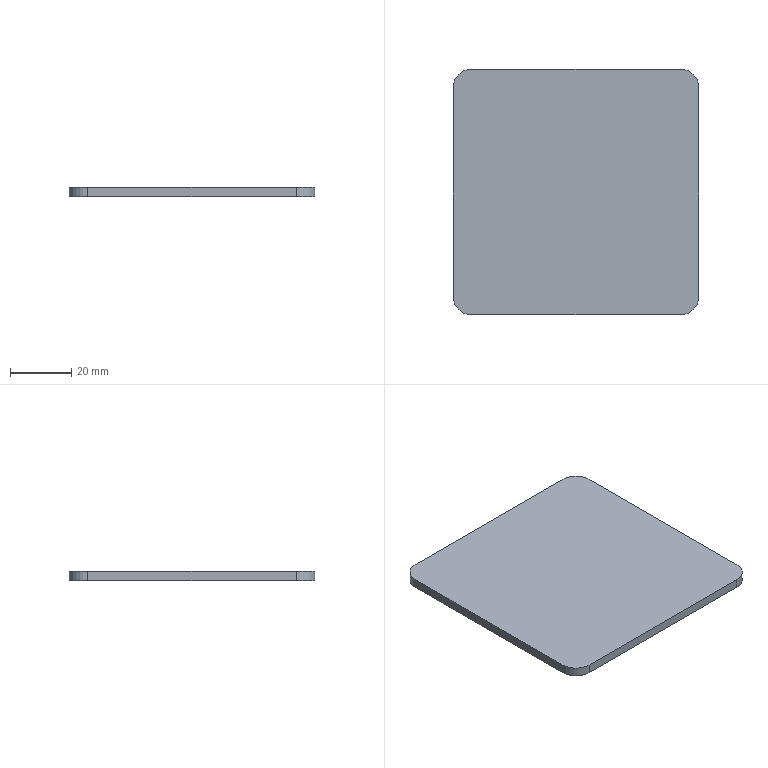Part | STEP file | SN10_008_006-04_TAMPA | 1 solid | 10 faces | box 80 x 80 x 3 mm | volume 19107 mm3 | plane 6 | cylinder 4 | commonest cylinder face diameters 12 x4
STEP:
#1=CARTESIAN_POINT('',(0.,0.,0.));
#2=DIRECTION('',(0.,0.,1.));
#3=DIRECTION('',(1.,0.,0.));
#4=AXIS2_PLACEMENT_3D('',#1,#2,#3);
#5=CARTESIAN_POINT('',(249.629,350.,449.));
#6=VERTEX_POINT('',#5);
#7=CARTESIAN_POINT('',(317.629,350.,449.));
#8=VERTEX_POINT('',#7);
#9=CARTESIAN_POINT('',(249.629,350.,449.));
#10=DIRECTION('',(1.,0.,0.));
#11=VECTOR('',#10,1.);
#12=LINE('',#9,#11);
#13=CARTESIAN_POINT('',(249.629,350.,446.));
#14=DIRECTION('',(0.,-1.,0.));
#15=DIRECTION('',(0.,0.,-1.));
#16=AXIS2_PLACEMENT_3D('',#13,#14,#15);
#17=PLANE('',#16);
#18=CARTESIAN_POINT('',(-3.,0.));
#19=DIRECTION('',(0.,1.));
#20=VECTOR('',#19,1.);
#21=LINE('',#18,#20);
#22=(GEOMETRIC_REPRESENTATION_CONTEXT(2)PARAMETRIC_REPRESENTATION_CONTEXT()REPRESENTATION_CONTEXT('',''));
#23=DEFINITIONAL_REPRESENTATION('',(#21),#22);
#24=PCURVE('',#17,#23);
#25=CARTESIAN_POINT('',(0.,0.,449.));
#26=DIRECTION('',(0.,0.,-1.));
#27=DIRECTION('',(-1.,0.,0.));
#28=AXIS2_PLACEMENT_3D('',#25,#26,#27);
#29=PLANE('',#28);
#30=CARTESIAN_POINT('',(-249.629,350.));
#31=DIRECTION('',(-1.,0.));
#32=VECTOR('',#31,1.);
#33=LINE('',#30,#32);
#34=(GEOMETRIC_REPRESENTATION_CONTEXT(2)PARAMETRIC_REPRESENTATION_CONTEXT()REPRESENTATION_CONTEXT('',''));
#35=DEFINITIONAL_REPRESENTATION('',(#33),#34);
#36=PCURVE('',#29,#35);
#37=SURFACE_CURVE('',#12,(#24,#36),.PCURVE_S1.);
#38=EDGE_CURVE('',#6,#8,#37,.T.);
#39=ORIENTED_EDGE('',*,*,#38,.T.);
#40=CARTESIAN_POINT('',(317.629,350.,446.));
#41=VERTEX_POINT('',#40);
#42=CARTESIAN_POINT('',(317.629,350.,446.));
#43=DIRECTION('',(0.,0.,1.));
#44=VECTOR('',#43,1.);
#45=LINE('',#42,#44);
#46=CARTESIAN_POINT('',(0.,68.));
#47=DIRECTION('',(-1.,0.));
#48=VECTOR('',#47,1.);
#49=LINE('',#46,#48);
#50=(GEOMETRIC_REPRESENTATION_CONTEXT(2)PARAMETRIC_REPRESENTATION_CONTEXT()REPRESENTATION_CONTEXT('',''));
#51=DEFINITIONAL_REPRESENTATION('',(#49),#50);
#52=PCURVE('',#17,#51);
#53=CARTESIAN_POINT('',(317.629,344.,447.5));
#54=DIRECTION('',(0.,0.,-1.));
#55=DIRECTION('',(0.,1.,0.));
#56=AXIS2_PLACEMENT_3D('',#53,#54,#55);
#57=CYLINDRICAL_SURFACE('',#56,6.);
#58=CARTESIAN_POINT('',(0.,1.5));
#59=DIRECTION('',(0.,-1.));
#60=VECTOR('',#59,1.);
#61=LINE('',#58,#60);
#62=(GEOMETRIC_REPRESENTATION_CONTEXT(2)PARAMETRIC_REPRESENTATION_CONTEXT()REPRESENTATION_CONTEXT('',''));
#63=DEFINITIONAL_REPRESENTATION('',(#61),#62);
#64=PCURVE('',#57,#63);
#65=SURFACE_CURVE('',#45,(#52,#64),.PCURVE_S1.);
#66=EDGE_CURVE('',#41,#8,#65,.T.);
#67=ORIENTED_EDGE('',*,*,#66,.F.);
#68=CARTESIAN_POINT('',(249.629,350.,446.));
#69=VERTEX_POINT('',#68);
#70=CARTESIAN_POINT('',(249.629,350.,446.));
#71=DIRECTION('',(1.,0.,0.));
#72=VECTOR('',#71,1.);
#73=LINE('',#70,#72);
#74=CARTESIAN_POINT('',(0.,0.));
#75=DIRECTION('',(0.,1.));
#76=VECTOR('',#75,1.);
#77=LINE('',#74,#76);
#78=(GEOMETRIC_REPRESENTATION_CONTEXT(2)PARAMETRIC_REPRESENTATION_CONTEXT()REPRESENTATION_CONTEXT('',''));
#79=DEFINITIONAL_REPRESENTATION('',(#77),#78);
#80=PCURVE('',#17,#79);
#81=CARTESIAN_POINT('',(0.,0.,446.));
#82=DIRECTION('',(0.,0.,-1.));
#83=DIRECTION('',(-1.,0.,0.));
#84=AXIS2_PLACEMENT_3D('',#81,#82,#83);
#85=PLANE('',#84);
#86=CARTESIAN_POINT('',(-249.629,350.));
#87=DIRECTION('',(-1.,0.));
#88=VECTOR('',#87,1.);
#89=LINE('',#86,#88);
#90=(GEOMETRIC_REPRESENTATION_CONTEXT(2)PARAMETRIC_REPRESENTATION_CONTEXT()REPRESENTATION_CONTEXT('',''));
#91=DEFINITIONAL_REPRESENTATION('',(#89),#90);
#92=PCURVE('',#85,#91);
#93=SURFACE_CURVE('',#73,(#80,#92),.PCURVE_S1.);
#94=EDGE_CURVE('',#69,#41,#93,.T.);
#95=ORIENTED_EDGE('',*,*,#94,.F.);
#96=CARTESIAN_POINT('',(249.629,350.,446.));
#97=DIRECTION('',(0.,0.,1.));
#98=VECTOR('',#97,1.);
#99=LINE('',#96,#98);
#100=CARTESIAN_POINT('',(0.,0.));
#101=DIRECTION('',(-1.,0.));
#102=VECTOR('',#101,1.);
#103=LINE('',#100,#102);
#104=(GEOMETRIC_REPRESENTATION_CONTEXT(2)PARAMETRIC_REPRESENTATION_CONTEXT()REPRESENTATION_CONTEXT('',''));
#105=DEFINITIONAL_REPRESENTATION('',(#103),#104);
#106=PCURVE('',#17,#105);
#107=CARTESIAN_POINT('',(249.629,344.,447.5));
#108=DIRECTION('',(0.,0.,-1.));
#109=DIRECTION('',(-1.,0.,0.));
#110=AXIS2_PLACEMENT_3D('',#107,#108,#109);
#111=CYLINDRICAL_SURFACE('',#110,6.);
#112=CARTESIAN_POINT('',(1.571,1.5));
#113=DIRECTION('',(0.,-1.));
#114=VECTOR('',#113,1.);
#115=LINE('',#112,#114);
#116=(GEOMETRIC_REPRESENTATION_CONTEXT(2)PARAMETRIC_REPRESENTATION_CONTEXT()REPRESENTATION_CONTEXT('',''));
#117=DEFINITIONAL_REPRESENTATION('',(#115),#116);
#118=PCURVE('',#111,#117);
#119=SURFACE_CURVE('',#99,(#106,#118),.PCURVE_S1.);
#120=EDGE_CURVE('',#69,#6,#119,.T.);
#121=ORIENTED_EDGE('',*,*,#120,.T.);
#122=EDGE_LOOP('',(#39,#67,#95,#121));
#123=FACE_BOUND('',#122,.T.);
#124=ADVANCED_FACE('',(#123),#17,.F.);
#125=CARTESIAN_POINT('',(323.629,344.,449.));
#126=VERTEX_POINT('',#125);
#127=CARTESIAN_POINT('',(317.629,344.,449.));
#128=DIRECTION('',(0.,0.,-1.));
#129=DIRECTION('',(1.,0.,0.));
#130=AXIS2_PLACEMENT_3D('',#127,#128,#129);
#131=CIRCLE('',#130,6.);
#132=CARTESIAN_POINT('',(-4.712,-1.5));
#133=DIRECTION('',(1.,0.));
#134=VECTOR('',#133,1.);
#135=LINE('',#132,#134);
#136=(GEOMETRIC_REPRESENTATION_CONTEXT(2)PARAMETRIC_REPRESENTATION_CONTEXT()REPRESENTATION_CONTEXT('',''));
#137=DEFINITIONAL_REPRESENTATION('',(#135),#136);
#138=PCURVE('',#57,#137);
#139=CARTESIAN_POINT('',(-317.629,344.));
#140=DIRECTION('',(-1.,0.));
#141=AXIS2_PLACEMENT_2D('',#139,#140);
#142=CIRCLE('',#141,6.);
#143=(GEOMETRIC_REPRESENTATION_CONTEXT(2)PARAMETRIC_REPRESENTATION_CONTEXT()REPRESENTATION_CONTEXT('',''));
#144=DEFINITIONAL_REPRESENTATION('',(#142),#143);
#145=PCURVE('',#29,#144);
#146=SURFACE_CURVE('',#131,(#138,#145),.PCURVE_S1.);
#147=EDGE_CURVE('',#8,#126,#146,.T.);
#148=ORIENTED_EDGE('',*,*,#147,.T.);
#149=CARTESIAN_POINT('',(323.629,344.,446.));
#150=VERTEX_POINT('',#149);
#151=CARTESIAN_POINT('',(323.629,344.,449.));
#152=DIRECTION('',(0.,0.,-1.));
#153=VECTOR('',#152,1.);
#154=LINE('',#151,#153);
#155=CARTESIAN_POINT('',(1.571,-1.5));
#156=DIRECTION('',(0.,1.));
#157=VECTOR('',#156,1.);
#158=LINE('',#155,#157);
#159=(GEOMETRIC_REPRESENTATION_CONTEXT(2)PARAMETRIC_REPRESENTATION_CONTEXT()REPRESENTATION_CONTEXT('',''));
#160=DEFINITIONAL_REPRESENTATION('',(#158),#159);
#161=PCURVE('',#57,#160);
#162=CARTESIAN_POINT('',(323.629,344.,446.));
#163=DIRECTION('',(-1.,0.,0.));
#164=DIRECTION('',(0.,0.,1.));
#165=AXIS2_PLACEMENT_3D('',#162,#163,#164);
#166=PLANE('',#165);
#167=CARTESIAN_POINT('',(3.,0.));
#168=DIRECTION('',(-1.,0.));
#169=VECTOR('',#168,1.);
#170=LINE('',#167,#169);
#171=(GEOMETRIC_REPRESENTATION_CONTEXT(2)PARAMETRIC_REPRESENTATION_CONTEXT()REPRESENTATION_CONTEXT('',''));
#172=DEFINITIONAL_REPRESENTATION('',(#170),#171);
#173=PCURVE('',#166,#172);
#174=SURFACE_CURVE('',#154,(#161,#173),.PCURVE_S1.);
#175=EDGE_CURVE('',#126,#150,#174,.T.);
#176=ORIENTED_EDGE('',*,*,#175,.T.);
#177=CARTESIAN_POINT('',(317.629,344.,446.));
#178=DIRECTION('',(0.,0.,-1.));
#179=DIRECTION('',(1.,0.,0.));
#180=AXIS2_PLACEMENT_3D('',#177,#178,#179);
#181=CIRCLE('',#180,6.);
#182=CARTESIAN_POINT('',(-4.712,1.5));
#183=DIRECTION('',(1.,0.));
#184=VECTOR('',#183,1.);
#185=LINE('',#182,#184);
#186=(GEOMETRIC_REPRESENTATION_CONTEXT(2)PARAMETRIC_REPRESENTATION_CONTEXT()REPRESENTATION_CONTEXT('',''));
#187=DEFINITIONAL_REPRESENTATION('',(#185),#186);
#188=PCURVE('',#57,#187);
#189=CARTESIAN_POINT('',(-317.629,344.));
#190=DIRECTION('',(-1.,0.));
#191=AXIS2_PLACEMENT_2D('',#189,#190);
#192=CIRCLE('',#191,6.);
#193=(GEOMETRIC_REPRESENTATION_CONTEXT(2)PARAMETRIC_REPRESENTATION_CONTEXT()REPRESENTATION_CONTEXT('',''));
#194=DEFINITIONAL_REPRESENTATION('',(#192),#193);
#195=PCURVE('',#85,#194);
#196=SURFACE_CURVE('',#181,(#188,#195),.PCURVE_S1.);
#197=EDGE_CURVE('',#41,#150,#196,.T.);
#198=ORIENTED_EDGE('',*,*,#197,.F.);
#199=ORIENTED_EDGE('',*,*,#66,.T.);
#200=EDGE_LOOP('',(#148,#176,#198,#199));
#201=FACE_BOUND('',#200,.T.);
#202=ADVANCED_FACE('',(#201),#57,.T.);
#203=CARTESIAN_POINT('',(323.629,276.,449.));
#204=VERTEX_POINT('',#203);
#205=CARTESIAN_POINT('',(323.629,344.,449.));
#206=DIRECTION('',(0.,-1.,0.));
#207=VECTOR('',#206,1.);
#208=LINE('',#205,#207);
#209=CARTESIAN_POINT('',(3.,0.));
#210=DIRECTION('',(0.,-1.));
#211=VECTOR('',#210,1.);
#212=LINE('',#209,#211);
#213=(GEOMETRIC_REPRESENTATION_CONTEXT(2)PARAMETRIC_REPRESENTATION_CONTEXT()REPRESENTATION_CONTEXT('',''));
#214=DEFINITIONAL_REPRESENTATION('',(#212),#213);
#215=PCURVE('',#166,#214);
#216=CARTESIAN_POINT('',(-323.629,344.));
#217=DIRECTION('',(0.,-1.));
#218=VECTOR('',#217,1.);
#219=LINE('',#216,#218);
#220=(GEOMETRIC_REPRESENTATION_CONTEXT(2)PARAMETRIC_REPRESENTATION_CONTEXT()REPRESENTATION_CONTEXT('',''));
#221=DEFINITIONAL_REPRESENTATION('',(#219),#220);
#222=PCURVE('',#29,#221);
#223=SURFACE_CURVE('',#208,(#215,#222),.PCURVE_S1.);
#224=EDGE_CURVE('',#126,#204,#223,.T.);
#225=ORIENTED_EDGE('',*,*,#224,.T.);
#226=CARTESIAN_POINT('',(323.629,276.,446.));
#227=VERTEX_POINT('',#226);
#228=CARTESIAN_POINT('',(323.629,276.,446.));
#229=DIRECTION('',(0.,0.,1.));
#230=VECTOR('',#229,1.);
#231=LINE('',#228,#230);
#232=CARTESIAN_POINT('',(0.,-68.));
#233=DIRECTION('',(1.,0.));
#234=VECTOR('',#233,1.);
#235=LINE('',#232,#234);
#236=(GEOMETRIC_REPRESENTATION_CONTEXT(2)PARAMETRIC_REPRESENTATION_CONTEXT()REPRESENTATION_CONTEXT('',''));
#237=DEFINITIONAL_REPRESENTATION('',(#235),#236);
#238=PCURVE('',#166,#237);
#239=CARTESIAN_POINT('',(317.629,276.,447.5));
#240=DIRECTION('',(0.,0.,-1.));
#241=DIRECTION('',(1.,0.,0.));
#242=AXIS2_PLACEMENT_3D('',#239,#240,#241);
#243=CYLINDRICAL_SURFACE('',#242,6.);
#244=CARTESIAN_POINT('',(0.,1.5));
#245=DIRECTION('',(0.,-1.));
#246=VECTOR('',#245,1.);
#247=LINE('',#244,#246);
#248=(GEOMETRIC_REPRESENTATION_CONTEXT(2)PARAMETRIC_REPRESENTATION_CONTEXT()REPRESENTATION_CONTEXT('',''));
#249=DEFINITIONAL_REPRESENTATION('',(#247),#248);
#250=PCURVE('',#243,#249);
#251=SURFACE_CURVE('',#231,(#238,#250),.PCURVE_S1.);
#252=EDGE_CURVE('',#227,#204,#251,.T.);
#253=ORIENTED_EDGE('',*,*,#252,.F.);
#254=CARTESIAN_POINT('',(323.629,344.,446.));
#255=DIRECTION('',(0.,-1.,0.));
#256=VECTOR('',#255,1.);
#257=LINE('',#254,#256);
#258=CARTESIAN_POINT('',(0.,0.));
#259=DIRECTION('',(0.,-1.));
#260=VECTOR('',#259,1.);
#261=LINE('',#258,#260);
#262=(GEOMETRIC_REPRESENTATION_CONTEXT(2)PARAMETRIC_REPRESENTATION_CONTEXT()REPRESENTATION_CONTEXT('',''));
#263=DEFINITIONAL_REPRESENTATION('',(#261),#262);
#264=PCURVE('',#166,#263);
#265=CARTESIAN_POINT('',(-323.629,344.));
#266=DIRECTION('',(0.,-1.));
#267=VECTOR('',#266,1.);
#268=LINE('',#265,#267);
#269=(GEOMETRIC_REPRESENTATION_CONTEXT(2)PARAMETRIC_REPRESENTATION_CONTEXT()REPRESENTATION_CONTEXT('',''));
#270=DEFINITIONAL_REPRESENTATION('',(#268),#269);
#271=PCURVE('',#85,#270);
#272=SURFACE_CURVE('',#257,(#264,#271),.PCURVE_S1.);
#273=EDGE_CURVE('',#150,#227,#272,.T.);
#274=ORIENTED_EDGE('',*,*,#273,.F.);
#275=ORIENTED_EDGE('',*,*,#175,.F.);
#276=EDGE_LOOP('',(#225,#253,#274,#275));
#277=FACE_BOUND('',#276,.T.);
#278=ADVANCED_FACE('',(#277),#166,.F.);
#279=CARTESIAN_POINT('',(317.629,270.,449.));
#280=VERTEX_POINT('',#279);
#281=CARTESIAN_POINT('',(317.629,276.,449.));
#282=DIRECTION('',(0.,0.,-1.));
#283=DIRECTION('',(1.,0.,0.));
#284=AXIS2_PLACEMENT_3D('',#281,#282,#283);
#285=CIRCLE('',#284,6.);
#286=CARTESIAN_POINT('',(0.,-1.5));
#287=DIRECTION('',(1.,0.));
#288=VECTOR('',#287,1.);
#289=LINE('',#286,#288);
#290=(GEOMETRIC_REPRESENTATION_CONTEXT(2)PARAMETRIC_REPRESENTATION_CONTEXT()REPRESENTATION_CONTEXT('',''));
#291=DEFINITIONAL_REPRESENTATION('',(#289),#290);
#292=PCURVE('',#243,#291);
#293=CARTESIAN_POINT('',(-317.629,276.));
#294=DIRECTION('',(-1.,0.));
#295=AXIS2_PLACEMENT_2D('',#293,#294);
#296=CIRCLE('',#295,6.);
#297=(GEOMETRIC_REPRESENTATION_CONTEXT(2)PARAMETRIC_REPRESENTATION_CONTEXT()REPRESENTATION_CONTEXT('',''));
#298=DEFINITIONAL_REPRESENTATION('',(#296),#297);
#299=PCURVE('',#29,#298);
#300=SURFACE_CURVE('',#285,(#292,#299),.PCURVE_S1.);
#301=EDGE_CURVE('',#204,#280,#300,.T.);
#302=ORIENTED_EDGE('',*,*,#301,.T.);
#303=CARTESIAN_POINT('',(317.629,270.,446.));
#304=VERTEX_POINT('',#303);
#305=CARTESIAN_POINT('',(317.629,270.,449.));
#306=DIRECTION('',(0.,0.,-1.));
#307=VECTOR('',#306,1.);
#308=LINE('',#305,#307);
#309=CARTESIAN_POINT('',(1.571,-1.5));
#310=DIRECTION('',(0.,1.));
#311=VECTOR('',#310,1.);
#312=LINE('',#309,#311);
#313=(GEOMETRIC_REPRESENTATION_CONTEXT(2)PARAMETRIC_REPRESENTATION_CONTEXT()REPRESENTATION_CONTEXT('',''));
#314=DEFINITIONAL_REPRESENTATION('',(#312),#313);
#315=PCURVE('',#243,#314);
#316=CARTESIAN_POINT('',(317.629,270.,446.));
#317=DIRECTION('',(0.,1.,0.));
#318=DIRECTION('',(0.,0.,1.));
#319=AXIS2_PLACEMENT_3D('',#316,#317,#318);
#320=PLANE('',#319);
#321=CARTESIAN_POINT('',(3.,0.));
#322=DIRECTION('',(-1.,0.));
#323=VECTOR('',#322,1.);
#324=LINE('',#321,#323);
#325=(GEOMETRIC_REPRESENTATION_CONTEXT(2)PARAMETRIC_REPRESENTATION_CONTEXT()REPRESENTATION_CONTEXT('',''));
#326=DEFINITIONAL_REPRESENTATION('',(#324),#325);
#327=PCURVE('',#320,#326);
#328=SURFACE_CURVE('',#308,(#315,#327),.PCURVE_S1.);
#329=EDGE_CURVE('',#280,#304,#328,.T.);
#330=ORIENTED_EDGE('',*,*,#329,.T.);
#331=CARTESIAN_POINT('',(317.629,276.,446.));
#332=DIRECTION('',(0.,0.,-1.));
#333=DIRECTION('',(1.,0.,0.));
#334=AXIS2_PLACEMENT_3D('',#331,#332,#333);
#335=CIRCLE('',#334,6.);
#336=CARTESIAN_POINT('',(0.,1.5));
#337=DIRECTION('',(1.,0.));
#338=VECTOR('',#337,1.);
#339=LINE('',#336,#338);
#340=(GEOMETRIC_REPRESENTATION_CONTEXT(2)PARAMETRIC_REPRESENTATION_CONTEXT()REPRESENTATION_CONTEXT('',''));
#341=DEFINITIONAL_REPRESENTATION('',(#339),#340);
#342=PCURVE('',#243,#341);
#343=CARTESIAN_POINT('',(-317.629,276.));
#344=DIRECTION('',(-1.,0.));
#345=AXIS2_PLACEMENT_2D('',#343,#344);
#346=CIRCLE('',#345,6.);
#347=(GEOMETRIC_REPRESENTATION_CONTEXT(2)PARAMETRIC_REPRESENTATION_CONTEXT()REPRESENTATION_CONTEXT('',''));
#348=DEFINITIONAL_REPRESENTATION('',(#346),#347);
#349=PCURVE('',#85,#348);
#350=SURFACE_CURVE('',#335,(#342,#349),.PCURVE_S1.);
#351=EDGE_CURVE('',#227,#304,#350,.T.);
#352=ORIENTED_EDGE('',*,*,#351,.F.);
#353=ORIENTED_EDGE('',*,*,#252,.T.);
#354=EDGE_LOOP('',(#302,#330,#352,#353));
#355=FACE_BOUND('',#354,.T.);
#356=ADVANCED_FACE('',(#355),#243,.T.);
#357=CARTESIAN_POINT('',(249.629,270.,449.));
#358=VERTEX_POINT('',#357);
#359=CARTESIAN_POINT('',(317.629,270.,449.));
#360=DIRECTION('',(-1.,0.,0.));
#361=VECTOR('',#360,1.);
#362=LINE('',#359,#361);
#363=CARTESIAN_POINT('',(3.,0.));
#364=DIRECTION('',(0.,-1.));
#365=VECTOR('',#364,1.);
#366=LINE('',#363,#365);
#367=(GEOMETRIC_REPRESENTATION_CONTEXT(2)PARAMETRIC_REPRESENTATION_CONTEXT()REPRESENTATION_CONTEXT('',''));
#368=DEFINITIONAL_REPRESENTATION('',(#366),#367);
#369=PCURVE('',#320,#368);
#370=CARTESIAN_POINT('',(-317.629,270.));
#371=DIRECTION('',(1.,0.));
#372=VECTOR('',#371,1.);
#373=LINE('',#370,#372);
#374=(GEOMETRIC_REPRESENTATION_CONTEXT(2)PARAMETRIC_REPRESENTATION_CONTEXT()REPRESENTATION_CONTEXT('',''));
#375=DEFINITIONAL_REPRESENTATION('',(#373),#374);
#376=PCURVE('',#29,#375);
#377=SURFACE_CURVE('',#362,(#369,#376),.PCURVE_S1.);
#378=EDGE_CURVE('',#280,#358,#377,.T.);
#379=ORIENTED_EDGE('',*,*,#378,.T.);
#380=CARTESIAN_POINT('',(249.629,270.,446.));
#381=VERTEX_POINT('',#380);
#382=CARTESIAN_POINT('',(249.629,270.,446.));
#383=DIRECTION('',(0.,0.,1.));
#384=VECTOR('',#383,1.);
#385=LINE('',#382,#384);
#386=CARTESIAN_POINT('',(0.,-68.));
#387=DIRECTION('',(1.,0.));
#388=VECTOR('',#387,1.);
#389=LINE('',#386,#388);
#390=(GEOMETRIC_REPRESENTATION_CONTEXT(2)PARAMETRIC_REPRESENTATION_CONTEXT()REPRESENTATION_CONTEXT('',''));
#391=DEFINITIONAL_REPRESENTATION('',(#389),#390);
#392=PCURVE('',#320,#391);
#393=CARTESIAN_POINT('',(249.629,276.,447.5));
#394=DIRECTION('',(0.,0.,-1.));
#395=DIRECTION('',(0.,-1.,0.));
#396=AXIS2_PLACEMENT_3D('',#393,#394,#395);
#397=CYLINDRICAL_SURFACE('',#396,6.);
#398=CARTESIAN_POINT('',(0.,1.5));
#399=DIRECTION('',(0.,-1.));
#400=VECTOR('',#399,1.);
#401=LINE('',#398,#400);
#402=(GEOMETRIC_REPRESENTATION_CONTEXT(2)PARAMETRIC_REPRESENTATION_CONTEXT()REPRESENTATION_CONTEXT('',''));
#403=DEFINITIONAL_REPRESENTATION('',(#401),#402);
#404=PCURVE('',#397,#403);
#405=SURFACE_CURVE('',#385,(#392,#404),.PCURVE_S1.);
#406=EDGE_CURVE('',#381,#358,#405,.T.);
#407=ORIENTED_EDGE('',*,*,#406,.F.);
#408=CARTESIAN_POINT('',(317.629,270.,446.));
#409=DIRECTION('',(-1.,0.,0.));
#410=VECTOR('',#409,1.);
#411=LINE('',#408,#410);
#412=CARTESIAN_POINT('',(0.,0.));
#413=DIRECTION('',(0.,-1.));
#414=VECTOR('',#413,1.);
#415=LINE('',#412,#414);
#416=(GEOMETRIC_REPRESENTATION_CONTEXT(2)PARAMETRIC_REPRESENTATION_CONTEXT()REPRESENTATION_CONTEXT('',''));
#417=DEFINITIONAL_REPRESENTATION('',(#415),#416);
#418=PCURVE('',#320,#417);
#419=CARTESIAN_POINT('',(-317.629,270.));
#420=DIRECTION('',(1.,0.));
#421=VECTOR('',#420,1.);
#422=LINE('',#419,#421);
#423=(GEOMETRIC_REPRESENTATION_CONTEXT(2)PARAMETRIC_REPRESENTATION_CONTEXT()REPRESENTATION_CONTEXT('',''));
#424=DEFINITIONAL_REPRESENTATION('',(#422),#423);
#425=PCURVE('',#85,#424);
#426=SURFACE_CURVE('',#411,(#418,#425),.PCURVE_S1.);
#427=EDGE_CURVE('',#304,#381,#426,.T.);
#428=ORIENTED_EDGE('',*,*,#427,.F.);
#429=ORIENTED_EDGE('',*,*,#329,.F.);
#430=EDGE_LOOP('',(#379,#407,#428,#429));
#431=FACE_BOUND('',#430,.T.);
#432=ADVANCED_FACE('',(#431),#320,.F.);
#433=CARTESIAN_POINT('',(243.629,276.,449.));
#434=VERTEX_POINT('',#433);
#435=CARTESIAN_POINT('',(249.629,276.,449.));
#436=DIRECTION('',(0.,0.,-1.));
#437=DIRECTION('',(1.,0.,0.));
#438=AXIS2_PLACEMENT_3D('',#435,#436,#437);
#439=CIRCLE('',#438,6.);
#440=CARTESIAN_POINT('',(-1.571,-1.5));
#441=DIRECTION('',(1.,0.));
#442=VECTOR('',#441,1.);
#443=LINE('',#440,#442);
#444=(GEOMETRIC_REPRESENTATION_CONTEXT(2)PARAMETRIC_REPRESENTATION_CONTEXT()REPRESENTATION_CONTEXT('',''));
#445=DEFINITIONAL_REPRESENTATION('',(#443),#444);
#446=PCURVE('',#397,#445);
#447=CARTESIAN_POINT('',(-249.629,276.));
#448=DIRECTION('',(-1.,0.));
#449=AXIS2_PLACEMENT_2D('',#447,#448);
#450=CIRCLE('',#449,6.);
#451=(GEOMETRIC_REPRESENTATION_CONTEXT(2)PARAMETRIC_REPRESENTATION_CONTEXT()REPRESENTATION_CONTEXT('',''));
#452=DEFINITIONAL_REPRESENTATION('',(#450),#451);
#453=PCURVE('',#29,#452);
#454=SURFACE_CURVE('',#439,(#446,#453),.PCURVE_S1.);
#455=EDGE_CURVE('',#358,#434,#454,.T.);
#456=ORIENTED_EDGE('',*,*,#455,.T.);
#457=CARTESIAN_POINT('',(243.629,276.,446.));
#458=VERTEX_POINT('',#457);
#459=CARTESIAN_POINT('',(243.629,276.,449.));
#460=DIRECTION('',(0.,0.,-1.));
#461=VECTOR('',#460,1.);
#462=LINE('',#459,#461);
#463=CARTESIAN_POINT('',(1.571,-1.5));
#464=DIRECTION('',(0.,1.));
#465=VECTOR('',#464,1.);
#466=LINE('',#463,#465);
#467=(GEOMETRIC_REPRESENTATION_CONTEXT(2)PARAMETRIC_REPRESENTATION_CONTEXT()REPRESENTATION_CONTEXT('',''));
#468=DEFINITIONAL_REPRESENTATION('',(#466),#467);
#469=PCURVE('',#397,#468);
#470=CARTESIAN_POINT('',(243.629,276.,446.));
#471=DIRECTION('',(1.,0.,0.));
#472=DIRECTION('',(0.,0.,-1.));
#473=AXIS2_PLACEMENT_3D('',#470,#471,#472);
#474=PLANE('',#473);
#475=CARTESIAN_POINT('',(-3.,0.));
#476=DIRECTION('',(1.,0.));
#477=VECTOR('',#476,1.);
#478=LINE('',#475,#477);
#479=(GEOMETRIC_REPRESENTATION_CONTEXT(2)PARAMETRIC_REPRESENTATION_CONTEXT()REPRESENTATION_CONTEXT('',''));
#480=DEFINITIONAL_REPRESENTATION('',(#478),#479);
#481=PCURVE('',#474,#480);
#482=SURFACE_CURVE('',#462,(#469,#481),.PCURVE_S1.);
#483=EDGE_CURVE('',#434,#458,#482,.T.);
#484=ORIENTED_EDGE('',*,*,#483,.T.);
#485=CARTESIAN_POINT('',(249.629,276.,446.));
#486=DIRECTION('',(0.,0.,-1.));
#487=DIRECTION('',(1.,0.,0.));
#488=AXIS2_PLACEMENT_3D('',#485,#486,#487);
#489=CIRCLE('',#488,6.);
#490=CARTESIAN_POINT('',(-1.571,1.5));
#491=DIRECTION('',(1.,0.));
#492=VECTOR('',#491,1.);
#493=LINE('',#490,#492);
#494=(GEOMETRIC_REPRESENTATION_CONTEXT(2)PARAMETRIC_REPRESENTATION_CONTEXT()REPRESENTATION_CONTEXT('',''));
#495=DEFINITIONAL_REPRESENTATION('',(#493),#494);
#496=PCURVE('',#397,#495);
#497=CARTESIAN_POINT('',(-249.629,276.));
#498=DIRECTION('',(-1.,0.));
#499=AXIS2_PLACEMENT_2D('',#497,#498);
#500=CIRCLE('',#499,6.);
#501=(GEOMETRIC_REPRESENTATION_CONTEXT(2)PARAMETRIC_REPRESENTATION_CONTEXT()REPRESENTATION_CONTEXT('',''));
#502=DEFINITIONAL_REPRESENTATION('',(#500),#501);
#503=PCURVE('',#85,#502);
#504=SURFACE_CURVE('',#489,(#496,#503),.PCURVE_S1.);
#505=EDGE_CURVE('',#381,#458,#504,.T.);
#506=ORIENTED_EDGE('',*,*,#505,.F.);
#507=ORIENTED_EDGE('',*,*,#406,.T.);
#508=EDGE_LOOP('',(#456,#484,#506,#507));
#509=FACE_BOUND('',#508,.T.);
#510=ADVANCED_FACE('',(#509),#397,.T.);
#511=CARTESIAN_POINT('',(243.629,344.,449.));
#512=VERTEX_POINT('',#511);
#513=CARTESIAN_POINT('',(243.629,276.,449.));
#514=DIRECTION('',(0.,1.,0.));
#515=VECTOR('',#514,1.);
#516=LINE('',#513,#515);
#517=CARTESIAN_POINT('',(-3.,0.));
#518=DIRECTION('',(0.,1.));
#519=VECTOR('',#518,1.);
#520=LINE('',#517,#519);
#521=(GEOMETRIC_REPRESENTATION_CONTEXT(2)PARAMETRIC_REPRESENTATION_CONTEXT()REPRESENTATION_CONTEXT('',''));
#522=DEFINITIONAL_REPRESENTATION('',(#520),#521);
#523=PCURVE('',#474,#522);
#524=CARTESIAN_POINT('',(-243.629,276.));
#525=DIRECTION('',(0.,1.));
#526=VECTOR('',#525,1.);
#527=LINE('',#524,#526);
#528=(GEOMETRIC_REPRESENTATION_CONTEXT(2)PARAMETRIC_REPRESENTATION_CONTEXT()REPRESENTATION_CONTEXT('',''));
#529=DEFINITIONAL_REPRESENTATION('',(#527),#528);
#530=PCURVE('',#29,#529);
#531=SURFACE_CURVE('',#516,(#523,#530),.PCURVE_S1.);
#532=EDGE_CURVE('',#434,#512,#531,.T.);
#533=ORIENTED_EDGE('',*,*,#532,.T.);
#534=CARTESIAN_POINT('',(243.629,344.,446.));
#535=VERTEX_POINT('',#534);
#536=CARTESIAN_POINT('',(243.629,344.,446.));
#537=DIRECTION('',(0.,0.,1.));
#538=VECTOR('',#537,1.);
#539=LINE('',#536,#538);
#540=CARTESIAN_POINT('',(0.,68.));
#541=DIRECTION('',(-1.,0.));
#542=VECTOR('',#541,1.);
#543=LINE('',#540,#542);
#544=(GEOMETRIC_REPRESENTATION_CONTEXT(2)PARAMETRIC_REPRESENTATION_CONTEXT()REPRESENTATION_CONTEXT('',''));
#545=DEFINITIONAL_REPRESENTATION('',(#543),#544);
#546=PCURVE('',#474,#545);
#547=CARTESIAN_POINT('',(0.,1.5));
#548=DIRECTION('',(0.,-1.));
#549=VECTOR('',#548,1.);
#550=LINE('',#547,#549);
#551=(GEOMETRIC_REPRESENTATION_CONTEXT(2)PARAMETRIC_REPRESENTATION_CONTEXT()REPRESENTATION_CONTEXT('',''));
#552=DEFINITIONAL_REPRESENTATION('',(#550),#551);
#553=PCURVE('',#111,#552);
#554=SURFACE_CURVE('',#539,(#546,#553),.PCURVE_S1.);
#555=EDGE_CURVE('',#535,#512,#554,.T.);
#556=ORIENTED_EDGE('',*,*,#555,.F.);
#557=CARTESIAN_POINT('',(243.629,276.,446.));
#558=DIRECTION('',(0.,1.,0.));
#559=VECTOR('',#558,1.);
#560=LINE('',#557,#559);
#561=CARTESIAN_POINT('',(0.,0.));
#562=DIRECTION('',(0.,1.));
#563=VECTOR('',#562,1.);
#564=LINE('',#561,#563);
#565=(GEOMETRIC_REPRESENTATION_CONTEXT(2)PARAMETRIC_REPRESENTATION_CONTEXT()REPRESENTATION_CONTEXT('',''));
#566=DEFINITIONAL_REPRESENTATION('',(#564),#565);
#567=PCURVE('',#474,#566);
#568=CARTESIAN_POINT('',(-243.629,276.));
#569=DIRECTION('',(0.,1.));
#570=VECTOR('',#569,1.);
#571=LINE('',#568,#570);
#572=(GEOMETRIC_REPRESENTATION_CONTEXT(2)PARAMETRIC_REPRESENTATION_CONTEXT()REPRESENTATION_CONTEXT('',''));
#573=DEFINITIONAL_REPRESENTATION('',(#571),#572);
#574=PCURVE('',#85,#573);
#575=SURFACE_CURVE('',#560,(#567,#574),.PCURVE_S1.);
#576=EDGE_CURVE('',#458,#535,#575,.T.);
#577=ORIENTED_EDGE('',*,*,#576,.F.);
#578=ORIENTED_EDGE('',*,*,#483,.F.);
#579=EDGE_LOOP('',(#533,#556,#577,#578));
#580=FACE_BOUND('',#579,.T.);
#581=ADVANCED_FACE('',(#580),#474,.F.);
#582=CARTESIAN_POINT('',(249.629,344.,449.));
#583=DIRECTION('',(0.,0.,-1.));
#584=DIRECTION('',(1.,0.,0.));
#585=AXIS2_PLACEMENT_3D('',#582,#583,#584);
#586=CIRCLE('',#585,6.);
#587=CARTESIAN_POINT('',(-3.142,-1.5));
#588=DIRECTION('',(1.,0.));
#589=VECTOR('',#588,1.);
#590=LINE('',#587,#589);
#591=(GEOMETRIC_REPRESENTATION_CONTEXT(2)PARAMETRIC_REPRESENTATION_CONTEXT()REPRESENTATION_CONTEXT('',''));
#592=DEFINITIONAL_REPRESENTATION('',(#590),#591);
#593=PCURVE('',#111,#592);
#594=CARTESIAN_POINT('',(-249.629,344.));
#595=DIRECTION('',(-1.,0.));
#596=AXIS2_PLACEMENT_2D('',#594,#595);
#597=CIRCLE('',#596,6.);
#598=(GEOMETRIC_REPRESENTATION_CONTEXT(2)PARAMETRIC_REPRESENTATION_CONTEXT()REPRESENTATION_CONTEXT('',''));
#599=DEFINITIONAL_REPRESENTATION('',(#597),#598);
#600=PCURVE('',#29,#599);
#601=SURFACE_CURVE('',#586,(#593,#600),.PCURVE_S1.);
#602=EDGE_CURVE('',#512,#6,#601,.T.);
#603=ORIENTED_EDGE('',*,*,#602,.T.);
#604=ORIENTED_EDGE('',*,*,#120,.F.);
#605=CARTESIAN_POINT('',(249.629,344.,446.));
#606=DIRECTION('',(0.,0.,-1.));
#607=DIRECTION('',(1.,0.,0.));
#608=AXIS2_PLACEMENT_3D('',#605,#606,#607);
#609=CIRCLE('',#608,6.);
#610=CARTESIAN_POINT('',(-3.142,1.5));
#611=DIRECTION('',(1.,0.));
#612=VECTOR('',#611,1.);
#613=LINE('',#610,#612);
#614=(GEOMETRIC_REPRESENTATION_CONTEXT(2)PARAMETRIC_REPRESENTATION_CONTEXT()REPRESENTATION_CONTEXT('',''));
#615=DEFINITIONAL_REPRESENTATION('',(#613),#614);
#616=PCURVE('',#111,#615);
#617=CARTESIAN_POINT('',(-249.629,344.));
#618=DIRECTION('',(-1.,0.));
#619=AXIS2_PLACEMENT_2D('',#617,#618);
#620=CIRCLE('',#619,6.);
#621=(GEOMETRIC_REPRESENTATION_CONTEXT(2)PARAMETRIC_REPRESENTATION_CONTEXT()REPRESENTATION_CONTEXT('',''));
#622=DEFINITIONAL_REPRESENTATION('',(#620),#621);
#623=PCURVE('',#85,#622);
#624=SURFACE_CURVE('',#609,(#616,#623),.PCURVE_S1.);
#625=EDGE_CURVE('',#535,#69,#624,.T.);
#626=ORIENTED_EDGE('',*,*,#625,.F.);
#627=ORIENTED_EDGE('',*,*,#555,.T.);
#628=EDGE_LOOP('',(#603,#604,#626,#627));
#629=FACE_BOUND('',#628,.T.);
#630=ADVANCED_FACE('',(#629),#111,.T.);
#631=ORIENTED_EDGE('',*,*,#94,.T.);
#632=ORIENTED_EDGE('',*,*,#197,.T.);
#633=ORIENTED_EDGE('',*,*,#273,.T.);
#634=ORIENTED_EDGE('',*,*,#351,.T.);
#635=ORIENTED_EDGE('',*,*,#427,.T.);
#636=ORIENTED_EDGE('',*,*,#505,.T.);
#637=ORIENTED_EDGE('',*,*,#576,.T.);
#638=ORIENTED_EDGE('',*,*,#625,.T.);
#639=EDGE_LOOP('',(#631,#632,#633,#634,#635,#636,#637,#638));
#640=FACE_BOUND('',#639,.T.);
#641=ADVANCED_FACE('',(#640),#85,.T.);
#642=ORIENTED_EDGE('',*,*,#602,.F.);
#643=ORIENTED_EDGE('',*,*,#532,.F.);
#644=ORIENTED_EDGE('',*,*,#455,.F.);
#645=ORIENTED_EDGE('',*,*,#378,.F.);
#646=ORIENTED_EDGE('',*,*,#301,.F.);
#647=ORIENTED_EDGE('',*,*,#224,.F.);
#648=ORIENTED_EDGE('',*,*,#147,.F.);
#649=ORIENTED_EDGE('',*,*,#38,.F.);
#650=EDGE_LOOP('',(#642,#643,#644,#645,#646,#647,#648,#649));
#651=FACE_BOUND('',#650,.T.);
#652=ADVANCED_FACE('',(#651),#29,.F.);
#653=CLOSED_SHELL('',(#124,#202,#278,#356,#432,#510,#581,#630,#641,#652));
#654=MANIFOLD_SOLID_BREP('',#653);
#655=(LENGTH_UNIT()NAMED_UNIT(*)SI_UNIT(.MILLI.,.METRE.));
#656=UNCERTAINTY_MEASURE_WITH_UNIT(LENGTH_MEASURE(0.0000001),#655,'','');
#657=(NAMED_UNIT(*)PLANE_ANGLE_UNIT()SI_UNIT($,.RADIAN.));
#658=(NAMED_UNIT(*)SI_UNIT($,.STERADIAN.)SOLID_ANGLE_UNIT());
#659=(GEOMETRIC_REPRESENTATION_CONTEXT(3)GLOBAL_UNCERTAINTY_ASSIGNED_CONTEXT((#656))GLOBAL_UNIT_ASSIGNED_CONTEXT((#655,#657,#658))REPRESENTATION_CONTEXT('',''));
#660=ADVANCED_BREP_SHAPE_REPRESENTATION('',(#4,#654),#659);